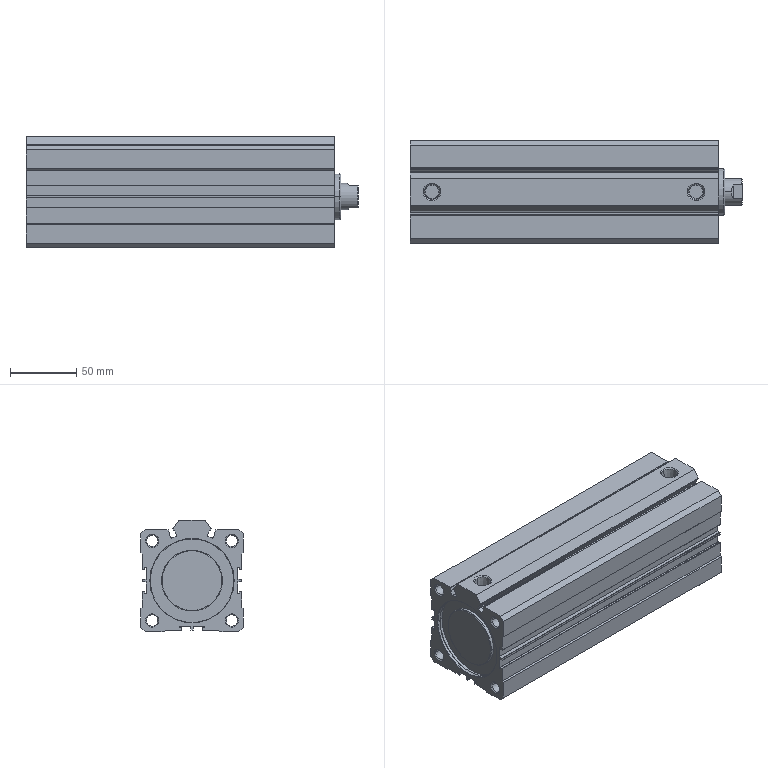Part | SolidWorks | 2 solids | 221 faces | box 250 x 77 x 84 mm | volume 780379 mm3 | plane 91 | cylinder 84 | cone 38 | torus 8 | commonest cylinder face diameters 0.4 x35 0.8 x15 8.376 x10 63 x8 20 x4 64 x4